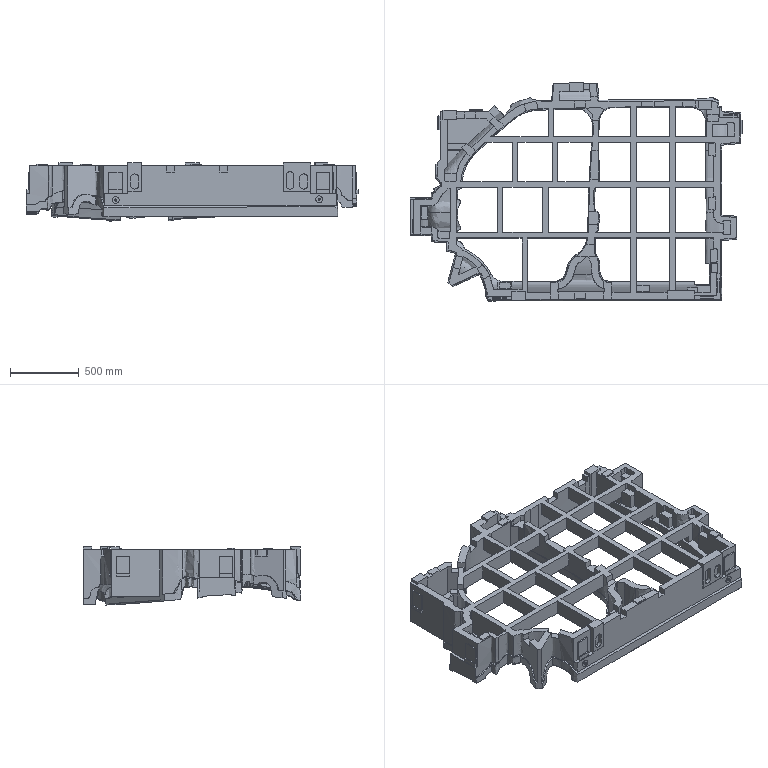Part | NX | features solid 2 | 1 solid | 1532 faces | box 2415 x 1585 x 422.73 mm | volume 241510120 mm3 | spline 986 | plane 456 | cylinder 82 | cone 8 | commonest cylinder face diameters 20 x24 52 x24 16 x9 50 x8 10 x3 10.001 x2